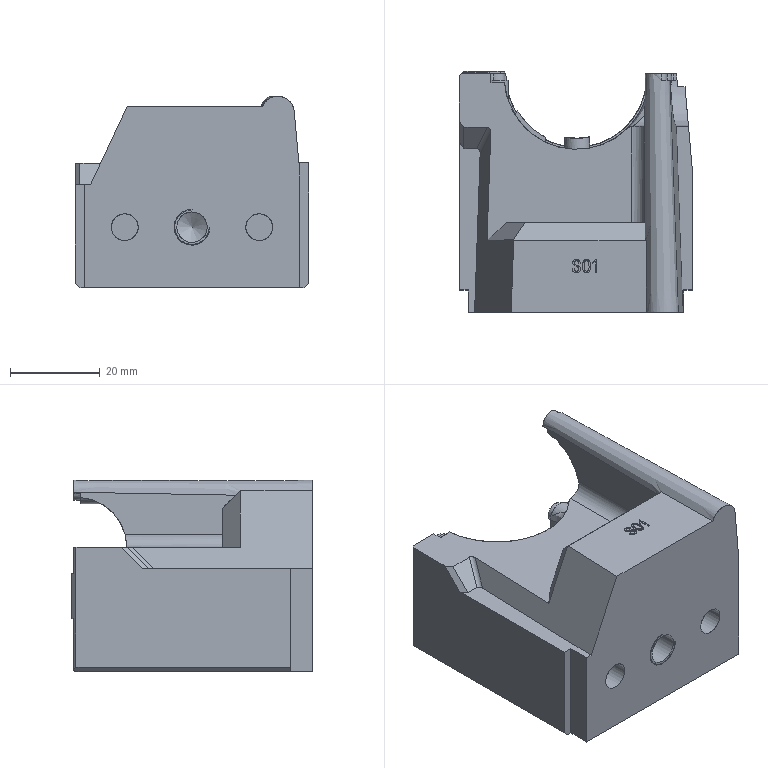NC program | PowerMill | posted with a generic post | part box 52 x 53.756 x 42.711 mm
Whole program:
%
O0001
N104 ( POWERMILL CB  : 2026004.0)
N105 ( POST VER      : 2026.0.0.5161)
N106 ( OPTION FILE   : FANUC)
N107 ( OUTPUT WORKPLANE : 1)
N108 (  )
N109 ( TOOL LIST )
N110 (--------------------------------)
N111 ( NO. | ID | DIA.| TIP RAD|LENGTH)
N112 (--------------------------------)
N113 (    1|D8_2| 8.0 |  0.0   | 99.0 )
N114 (--------------------------------)
N115 (  )
N116 ( NUMBER OF TOOLPATHS: 1.0 )
N117 ( ESTIMATED PROGRAM DURATION: 0 HOURS 1 MIN 35 SEC)
N118 (  )
N119 G00 G21 G80 G40 G17
N120 G90
N121 G54
N122 G53 Z0.0
N123 (---------------)
N124 ( START TOOLPATH : 02开粗-D8-等高 )
N125 (---------------)
N126 ( TOOL NO.    :1 )
N127 ( TOOL TYPE   : ENDMILL)
N128 ( TOOL ID     : D8_2)
N129 ( TOOL DIA    : 8.0 LENGTH 99.0)
N130 T1
N131 M6
N132 S3500 M03
N133 G00 G90 X28.2444 Y-5.4315
N134 G43 Z20.0 H1
N135
N136 G05 P10000 R8
N137 Z2.8808
N138 G01 Z-0.1192 F1680.0
N139 G02 X28.03 Y-4.6315 I1.3856 J0.8 F2800.0
N140 G01 Y0.1685
N141 Y42.5415
N142 Y47.3415
N143 G02 X28.2443 Y48.1415 I1.6 J0.0
N144 G01 X28.2654 Y48.178 Z-0.1366
N145 X28.2741 Y48.1931 Z-0.1788
N146 X28.2654 Y48.178 Z-0.2209
N147 X28.2443 Y48.1415 Z-0.2384
N148 G03 X28.03 Y47.3415 I1.3857 J-0.8
N149 G01 Y42.5415
N150 Y0.1685
N151 Y-4.6315
N152 G03 X28.2444 Y-5.4315 I1.6 J0.0
N153 G01 X28.2654 Y-5.468 Z-0.2558
N154 X28.2742 Y-5.4832 Z-0.298
N155 X28.2654 Y-5.468 Z-0.3401
N156 X28.2444 Y-5.4315 Z-0.3576
N157 G02 X28.03 Y-4.6315 I1.3856 J0.8
N158 G01 Y0.1685
N159 Y42.5415
N160 Y47.3415
N161 G02 X28.2443 Y48.1415 I1.6 J0.0
N162 G01 X28.2654 Y48.178 Z-0.375
N163 X28.2741 Y48.1931 Z-0.4172
N164 X28.2654 Y48.178 Z-0.4593
N165 X28.2443 Y48.1415 Z-0.4768
N166 G03 X28.03 Y47.3415 I1.3857 J-0.8
N167 G01 Y42.5415
N168 Y0.1685
N169 Y-4.6315
N170 G03 X28.2444 Y-5.4315 I1.6 J0.0
N171 G01 X28.2654 Y-5.468 Z-0.4942
N172 X28.2742 Y-5.4832 Z-0.5364
N173 X28.2654 Y-5.468 Z-0.5785
N174 X28.2444 Y-5.4315 Z-0.596
N175 G02 X28.03 Y-4.6315 I1.3856 J0.8
N176 G01 Y0.1685
N177 Y42.5415
N178 Y47.3415
N179 G02 X28.2443 Y48.1415 I1.6 J0.0
N180 G01 X28.2654 Y48.178 Z-0.6134
N181 X28.2741 Y48.1931 Z-0.6555
N182 X28.2654 Y48.178 Z-0.6977
N183 X28.2443 Y48.1415 Z-0.7151
N184 G03 X28.03 Y47.3415 I1.3857 J-0.8
N185 G01 Y42.5415
N186 Y0.1685
N187 Y-4.6315
N188 G03 X28.2444 Y-5.4315 I1.6 J0.0
N189 G01 X28.2654 Y-5.468 Z-0.7326
N190 X28.2742 Y-5.4832 Z-0.7747
N191 X28.2654 Y-5.468 Z-0.8169
N192 X28.2444 Y-5.4315 Z-0.8343
N193 G02 X28.03 Y-4.6315 I1.3856 J0.8
N194 G01 Y0.1685
N195 Y42.5415
N196 Y47.3415
N197 G02 X28.2443 Y48.1415 I1.6 J0.0
N198 G01 X28.2654 Y48.178 Z-0.8518
N199 X28.2741 Y48.1931 Z-0.8939
N200 X28.2654 Y48.178 Z-0.9361
N201 X28.2443 Y48.1415 Z-0.9535
N202 G03 X28.03 Y47.3415 I1.3857 J-0.8
N203 G01 Y42.5415
N204 Y0.1685
N205 Y-4.6315
N206 G03 X28.2444 Y-5.4315 I1.6 J0.0
N207 G01 X28.2654 Y-5.468 Z-0.971
N208 X28.2742 Y-5.4832 Z-1.0131
N209 X28.2654 Y-5.468 Z-1.0553
N210 X28.2444 Y-5.4315 Z-1.0727
N211 G02 X28.03 Y-4.6315 I1.3856 J0.8
N212 G01 Y0.1685
N213 Y42.5415
N214 Y47.3415
N215 G02 X28.2443 Y48.1415 I1.6 J0.0
N216 G01 X28.2654 Y48.178 Z-1.0902
N217 X28.2741 Y48.1931 Z-1.1323
N218 X28.2654 Y48.178 Z-1.1745
N219 X28.2443 Y48.1415 Z-1.1919
N220 G03 X28.03 Y47.3415 I1.3857 J-0.8
N221 G01 Y42.5415
N222 Y0.1685
N223 Y-4.6315
N224 G03 X28.2444 Y-5.4315 I1.6 J0.0
N225 G01 X28.2654 Y-5.468 Z-1.2094
N226 X28.2742 Y-5.4832 Z-1.2515
N227 X28.2654 Y-5.468 Z-1.2936
N228 X28.2444 Y-5.4315 Z-1.3111
N229 G02 X28.03 Y-4.6315 I1.3856 J0.8
N230 G01 Y0.1685
N231 Y42.5415
N232 Y47.3415
N233 G02 X28.2443 Y48.1415 I1.6 J0.0
N234 G01 X28.2654 Y48.178 Z-1.3285
N235 X28.2741 Y48.1931 Z-1.3707
N236 X28.2654 Y48.178 Z-1.4128
N237 X28.2443 Y48.1415 Z-1.4303
N238 G03 X28.03 Y47.3415 I1.3857 J-0.8
N239 G01 Y42.5415
N240 Y0.1685
N241 Y-4.6315
N242 G03 X28.2444 Y-5.4315 I1.6 J0.0
N243 G01 X28.2654 Y-5.468 Z-1.4477
N244 X28.2742 Y-5.4832 Z-1.4899
N245 X28.2654 Y-5.468 Z-1.532
N246 X28.2444 Y-5.4315 Z-1.5495
N247 G02 X28.03 Y-4.6315 I1.3856 J0.8
N248 G01 Y0.1685
N249 Y42.5415
N250 Y47.3415
N251 G02 X28.2443 Y48.1415 I1.6 J0.0
N252 G01 X28.2654 Y48.178 Z-1.5669
N253 X28.2741 Y48.1931 Z-1.6091
N254 X28.2654 Y48.178 Z-1.6512
N255 X28.2443 Y48.1415 Z-1.6687
N256 G03 X28.03 Y47.3415 I1.3857 J-0.8
N257 G01 Y42.5415
N258 Y0.1685
N259 Y-4.6315
N260 G03 X28.2444 Y-5.4315 I1.6 J0.0
N261 G01 X28.2654 Y-5.468 Z-1.6861
N262 X28.2742 Y-5.4832 Z-1.7283
N263 X28.2654 Y-5.468 Z-1.7704
N264 X28.2444 Y-5.4315 Z-1.7879
N265 G02 X28.03 Y-4.6315 I1.3856 J0.8
N266 G01 Y0.1685
N267 Y42.5415
N268 Y47.3415
N269 G02 X28.2443 Y48.1415 I1.6 J0.0
N270 G01 X28.2654 Y48.178 Z-1.8053
N271 X28.2741 Y48.1931 Z-1.8475
N272 X28.2654 Y48.178 Z-1.8896
N273 X28.2443 Y48.1415 Z-1.907
N274 G03 X28.03 Y47.3415 I1.3857 J-0.8
N275 G01 Y42.5415
N276 Y0.1685
N277 Y-4.6315
N278 G03 X28.2444 Y-5.4315 I1.6 J0.0
N279 G01 X28.2654 Y-5.468 Z-1.9245
N280 X28.2742 Y-5.4832 Z-1.9666
N281 X28.2654 Y-5.468 Z-2.0088
N282 X28.2444 Y-5.4315 Z-2.0262
N283 G02 X28.03 Y-4.6315 I1.3856 J0.8
N284 G01 Y0.1685
N285 Y42.5415
N286 Y47.3415
N287 G02 X28.2443 Y48.1415 I1.6 J0.0
N288 G01 X28.2654 Y48.178 Z-2.0437
N289 X28.2741 Y48.1931 Z-2.0858
N290 X28.2654 Y48.178 Z-2.128
N291 X28.2443 Y48.1415 Z-2.1454
N292 G03 X28.03 Y47.3415 I1.3857 J-0.8
N293 G01 Y42.5415
N294 Y0.1685
N295 Y-4.6315
N296 G03 X28.2444 Y-5.4315 I1.6 J0.0
N297 G01 X28.2654 Y-5.468 Z-2.1629
N298 X28.2742 Y-5.4832 Z-2.205
N299 X28.2654 Y-5.468 Z-2.2472
N300 X28.2444 Y-5.4315 Z-2.2646
N301 G02 X28.03 Y-4.6315 I1.3856 J0.8
N302 G01 Y0.1685
N303 Y42.5415
N304 Y47.3415
N305 G02 X28.2443 Y48.1415 I1.6 J0.0
N306 G01 X28.2654 Y48.178 Z-2.2821
N307 X28.2741 Y48.1931 Z-2.3242
N308 X28.2654 Y48.178 Z-2.3664
N309 X28.2443 Y48.1415 Z-2.3838
N310 G03 X28.03 Y47.3415 I1.3857 J-0.8
N311 G01 Y42.5415
N312 Y0.1685
N313 Y-4.6315
N314 G03 X28.2444 Y-5.4315 I1.6 J0.0
N315 G01 X28.2654 Y-5.468 Z-2.4013
N316 X28.2742 Y-5.4832 Z-2.4434
N317 X28.2655 Y-5.468 Z-2.4855
N318 X28.2444 Y-5.4315 Z-2.503
N319 G02 X28.03 Y-4.6315 I1.3856 J0.8
N320 G01 Y0.1685
N321 Y42.5415
N322 Y47.3415
N323 G02 X28.2443 Y48.1415 I1.6 J0.0
N324 G01 X28.2654 Y48.178 Z-2.5205
N325 X28.2741 Y48.1931 Z-2.5626
N326 X28.2654 Y48.178 Z-2.6047
N327 X28.2443 Y48.1415 Z-2.6222
N328 G03 X28.03 Y47.3415 I1.3857 J-0.8
N329 G01 Y42.5415
N330 Y0.1685
N331 Y-4.6315
N332 G03 X28.2444 Y-5.4315 I1.6 J0.0
N333 G01 X28.2655 Y-5.468 Z-2.6396
N334 X28.2742 Y-5.4832 Z-2.6818
N335 X28.2655 Y-5.468 Z-2.7239
N336 X28.2444 Y-5.4315 Z-2.7414
N337 G02 X28.03 Y-4.6315 I1.3856 J0.8
N338 G01 Y0.1685
N339 Y42.5415
N340 Y47.3415
N341 G02 X28.2444 Y48.1415 I1.6 J0.0
N342 G01 X28.2654 Y48.178 Z-2.7588
N343 X28.2741 Y48.1931 Z-2.801
N344 X28.2654 Y48.178 Z-2.8431
N345 X28.2444 Y48.1415 Z-2.8606
N346 G03 X28.03 Y47.3415 I1.3856 J-0.8
N347 G01 Y42.5415
N348 Y0.1685
N349 Y-4.6315
N350 G03 X28.2444 Y-5.4315 I1.6 J0.0
N351 G01 X28.2655 Y-5.468 Z-2.878
N352 X28.2742 Y-5.4832 Z-2.9202
N353 X28.2655 Y-5.468 Z-2.9623
N354 X28.2444 Y-5.4315 Z-2.9798
N355 G02 X28.03 Y-4.6315 I1.3856 J0.8
N356 G01 Y0.1685
N357 Y42.5415
N358 Y47.3415
N359 G02 X28.2444 Y48.1415 I1.6 J0.0
N360 G01 X28.2654 Y48.178 Z-2.9972
N361 X28.2742 Y48.1931 Z-3.0394
N362 X28.2654 Y48.178 Z-3.0815
N363 X28.2444 Y48.1415 Z-3.099
N364 G03 X28.03 Y47.3415 I1.3856 J-0.8
N365 G01 Y42.5415
N366 Y0.1685
N367 Y-4.6315
N368 G03 X28.2444 Y-5.4315 I1.6 J0.0
N369 G01 X28.2655 Y-5.468 Z-3.1164
N370 X28.2742 Y-5.4832 Z-3.1585
N371 X28.2655 Y-5.468 Z-3.2007
N372 X28.2444 Y-5.4315 Z-3.2181
N373 G02 X28.03 Y-4.6315 I1.3856 J0.8
N374 G01 Y0.1685
N375 Y42.5415
N376 Y47.3415
N377 G02 X28.2444 Y48.1415 I1.6 J0.0
N378 G01 X28.2654 Y48.178 Z-3.2356
N379 X28.2742 Y48.1932 Z-3.2777
N380 X28.2654 Y48.178 Z-3.3199
N381 X28.2444 Y48.1415 Z-3.3373
N382 G03 X28.03 Y47.3415 I1.3856 J-0.8
N383 G01 Y42.5415
N384 Y0.1685
N385 Y-4.6315
N386 G03 X28.2444 Y-5.4315 I1.6 J0.0
N387 G01 X28.2655 Y-5.468 Z-3.3548
N388 X28.2742 Y-5.4832 Z-3.3969
N389 X28.2655 Y-5.468 Z-3.4391
N390 X28.2444 Y-5.4315 Z-3.4565
N391 G02 X28.03 Y-4.6315 I1.3856 J0.8
N392 G01 Y0.1685
N393 Y42.5415
N394 Y47.3415
N395 G02 X28.2444 Y48.1415 I1.6 J0.0
N396 G01 X28.2654 Y48.178 Z-3.474
N397 X28.2742 Y48.1931 Z-3.5161
N398 X28.2654 Y48.178 Z-3.5583
N399 X28.2444 Y48.1415 Z-3.5757
N400 G03 X28.03 Y47.3415 I1.3856 J-0.8
N401 G01 Y42.5415
N402 Y0.1685
N403 Y-4.6315
N404 G03 X28.2444 Y-5.4315 I1.6 J0.0
N405 G01 X28.2655 Y-5.468 Z-3.5932
N406 X28.2742 Y-5.4832 Z-3.6353
N407 X28.2655 Y-5.468 Z-3.6774
N408 X28.2444 Y-5.4315 Z-3.6949
N409 G02 X28.03 Y-4.6315 I1.3856 J0.8
N410 G01 Y0.1685
N411 Y42.5415
N412 Y47.3415
N413 G02 X28.2444 Y48.1415 I1.6 J0.0
N414 G01 X28.2654 Y48.178 Z-3.7124
N415 X28.2742 Y48.1931 Z-3.7545
N416 X28.2654 Y48.178 Z-3.7966
N417 X28.2444 Y48.1415 Z-3.8141
N418 G03 X28.03 Y47.3415 I1.3856 J-0.8
N419 G01 Y42.5415
N420 Y0.1685
N421 Y-4.6315
N422 G03 X28.2444 Y-5.4315 I1.6 J0.0
N423 G01 X28.2655 Y-5.468 Z-3.8316
N424 X28.2742 Y-5.4832 Z-3.8737
N425 X28.2655 Y-5.468 Z-3.9158
N426 X28.2444 Y-5.4315 Z-3.9333
N427 G02 X28.03 Y-4.6315 I1.3856 J0.8
N428 G01 Y0.1685
N429 Y42.5415
N430 Y47.3415
N431 G02 X28.2444 Y48.1415 I1.6 J0.0
N432 G01 X28.2654 Y48.178 Z-3.9507
N433 X28.2742 Y48.1932 Z-3.9929
N434 X28.2654 Y48.178 Z-4.035
N435 X28.2444 Y48.1415 Z-4.0525
N436 G03 X28.03 Y47.3415 I1.3856 J-0.8
N437 G01 Y42.5415
N438 Y0.1685
N439 Y-4.6315
N440 G03 X28.2444 Y-5.4315 I1.6 J0.0
N441 G01 X28.2655 Y-5.468 Z-4.0699
N442 X28.2742 Y-5.4832 Z-4.1121
N443 X28.2655 Y-5.468 Z-4.1542
N444 X28.2444 Y-5.4315 Z-4.1717
N445 G02 X28.03 Y-4.6315 I1.3856 J0.8
N446 G01 Y0.1685
N447 Y42.5415
N448 Y47.3415
N449 G02 X28.2444 Y48.1415 I1.6 J0.0
N450 G01 X28.2654 Y48.178 Z-4.1891
N451 X28.2742 Y48.1932 Z-4.2313
N452 X28.2654 Y48.178 Z-4.2734
N453 X28.2444 Y48.1415 Z-4.2909
N454 G03 X28.03 Y47.3415 I1.3856 J-0.8
N455 G01 Y42.5415
N456 Y0.1685
N457 Y-4.6315
N458 G03 X28.2444 Y-5.4315 I1.6 J0.0
N459 G01 X28.2655 Y-5.468 Z-4.3083
N460 X28.2742 Y-5.4832 Z-4.3505
N461 X28.2655 Y-5.468 Z-4.3926
N462 X28.2444 Y-5.4315 Z-4.41
N463 G02 X28.03 Y-4.6315 I1.3856 J0.8
N464 G01 Y0.1685
N465 Y42.5415
N466 Y47.3415
N467 G02 X28.2444 Y48.1415 I1.6 J0.0
N468 G01 X28.2654 Y48.178 Z-4.4275
N469 X28.2742 Y48.1932 Z-4.4696
N470 X28.2654 Y48.178 Z-4.5118
N471 X28.2444 Y48.1415 Z-4.5292
N472 G03 X28.03 Y47.3415 I1.3856 J-0.8
N473 G01 Y42.5415
N474 Y0.1685
N475 Y-4.6315
N476 G03 X28.2444 Y-5.4315 I1.6 J0.0
N477 G01 X28.2655 Y-5.468 Z-4.5467
N478 X28.2742 Y-5.4832 Z-4.5888
N479 X28.2655 Y-5.468 Z-4.631
N480 X28.2444 Y-5.4315 Z-4.6484
N481 G02 X28.03 Y-4.6315 I1.3856 J0.8
N482 G01 Y0.1685
N483 Y42.5415
N484 Y47.3415
N485 G02 X28.2444 Y48.1415 I1.6 J0.0
N486 G01 X28.2654 Y48.178 Z-4.6659
N487 X28.2742 Y48.1932 Z-4.708
N488 X28.2654 Y48.178 Z-4.7502
N489 X28.2444 Y48.1415 Z-4.7676
N490 G03 X28.03 Y47.3415 I1.3856 J-0.8
N491 G01 Y42.5415
N492 Y0.1685
N493 Y-4.6315
N494 G03 X28.2444 Y-5.4315 I1.6 J0.0
N495 G01 X28.2655 Y-5.468 Z-4.7851
N496 X28.2742 Y-5.4832 Z-4.8272
N497 X28.2655 Y-5.468 Z-4.8694
N498 X28.2444 Y-5.4315 Z-4.8868
N499 G02 X28.03 Y-4.6315 I1.3856 J0.8
N500 G01 Y0.1685
N501 Y42.5415
N502 Y47.3415
N503 G02 X28.2444 Y48.1415 I1.6 J0.0
N504 G00 Z5.2882
N505 G01 X-28.2443 Y-5.4315 F10000.0
N506 G00 Z2.8808
N507 G01 Z-0.1192 F1680.0
N508 G03 X-28.03 Y-4.6315 I-1.3857 J0.8 F2800.0
N509 G01 Y0.1685
N510 Y42.5415
N511 Y47.3415
N512 G03 X-28.2443 Y48.1415 I-1.5999 J0.0001
N513 G01 X-28.2654 Y48.178 Z-0.1366
N514 X-28.2741 Y48.1931 Z-0.1788
N515 X-28.2654 Y48.178 Z-0.2209
N516 X-28.2443 Y48.1415 Z-0.2384
N517 G02 X-28.03 Y47.3415 I-1.3856 J-0.7999
N518 G01 Y42.5415
N519 Y0.1685
N520 Y-4.6315
N521 G02 X-28.2443 Y-5.4315 I-1.6 J0.0
N522 G01 X-28.2654 Y-5.468 Z-0.2558
N523 X-28.2741 Y-5.4832 Z-0.298
N524 X-28.2654 Y-5.468 Z-0.3401
N525 X-28.2443 Y-5.4315 Z-0.3576
N526 G03 X-28.03 Y-4.6315 I-1.3857 J0.8
N527 G01 Y0.1685
N528 Y42.5415
N529 Y47.3415
N530 G03 X-28.2443 Y48.1415 I-1.5999 J0.0001
N531 G01 X-28.2654 Y48.178 Z-0.375
N532 X-28.2741 Y48.1931 Z-0.4172
N533 X-28.2654 Y48.178 Z-0.4593
N534 X-28.2443 Y48.1415 Z-0.4768
N535 G02 X-28.03 Y47.3415 I-1.3856 J-0.7999
N536 G01 Y42.5415
N537 Y0.1685
N538 Y-4.6315
N539 G02 X-28.2443 Y-5.4315 I-1.6 J0.0
N540 G01 X-28.2654 Y-5.468 Z-0.4942
N541 X-28.2741 Y-5.4832 Z-0.5364
N542 X-28.2654 Y-5.468 Z-0.5785
N543 X-28.2443 Y-5.4315 Z-0.596
N544 G03 X-28.03 Y-4.6315 I-1.3857 J0.8
N545 G01 Y0.1685
N546 Y42.5415
N547 Y47.3415
N548 G03 X-28.2443 Y48.1415 I-1.5999 J0.0001
N549 G01 X-28.2654 Y48.178 Z-0.6134
N550 X-28.2741 Y48.1931 Z-0.6555
N551 X-28.2654 Y48.178 Z-0.6977
N552 X-28.2443 Y48.1415 Z-0.7151
N553 G02 X-28.03 Y47.3415 I-1.3856 J-0.7999
N554 G01 Y42.5415
N555 Y0.1685
N556 Y-4.6315
N557 G02 X-28.2443 Y-5.4315 I-1.6 J0.0
N558 G01 X-28.2654 Y-5.468 Z-0.7326
N559 X-28.2741 Y-5.4832 Z-0.7747
N560 X-28.2654 Y-5.468 Z-0.8169
N561 X-28.2443 Y-5.4315 Z-0.8343
N562 G03 X-28.03 Y-4.6315 I-1.3857 J0.8
N563 G01 Y0.1685
N564 Y42.5415
N565 Y47.3415
N566 G03 X-28.2443 Y48.1415 I-1.5999 J0.0001
N567 G01 X-28.2654 Y48.178 Z-0.8518
N568 X-28.2741 Y48.1931 Z-0.8939
N569 X-28.2654 Y48.178 Z-0.9361
N570 X-28.2443 Y48.1415 Z-0.9535
N571 G02 X-28.03 Y47.3415 I-1.3856 J-0.7999
N572 G01 Y42.5415
N573 Y0.1685
N574 Y-4.6315
N575 G02 X-28.2443 Y-5.4315 I-1.6 J0.0
N576 G01 X-28.2654 Y-5.468 Z-0.971
N577 X-28.2741 Y-5.4832 Z-1.0131
N578 X-28.2654 Y-5.468 Z-1.0553
N579 X-28.2443 Y-5.4315 Z-1.0727
N580 G03 X-28.03 Y-4.6315 I-1.3857 J0.8
N581 G01 Y0.1685
N582 Y42.5415
N583 Y47.3415
N584 G03 X-28.2443 Y48.1415 I-1.5999 J0.0001
N585 G01 X-28.2654 Y48.178 Z-1.0902
N586 X-28.2741 Y48.1931 Z-1.1323
N587 X-28.2654 Y48.178 Z-1.1745
N588 X-28.2443 Y48.1415 Z-1.1919
N589 G02 X-28.03 Y47.3415 I-1.3856 J-0.7999
N590 G01 Y42.5415
N591 Y0.1685
N592 Y-4.6315
N593 G02 X-28.2443 Y-5.4315 I-1.6 J0.0
N594 G01 X-28.2654 Y-5.468 Z-1.2094
N595 X-28.2741 Y-5.4832 Z-1.2515
N596 X-28.2654 Y-5.468 Z-1.2936
N597 X-28.2444 Y-5.4315 Z-1.3111
N598 G03 X-28.03 Y-4.6315 I-1.3856 J0.8
N599 G01 Y0.1685
N600 Y42.5415
N601 Y47.3415
N602 G03 X-28.2444 Y48.1415 I-1.5999 J0.0001
N603 G01 X-28.2654 Y48.178 Z-1.3285
N604 X-28.2741 Y48.1931 Z-1.3707
N605 X-28.2654 Y48.178 Z-1.4128
N606 X-28.2444 Y48.1415 Z-1.4303
N607 G02 X-28.03 Y47.3415 I-1.3855 J-0.7999
N608 G01 Y42.5415
N609 Y0.1685
N610 Y-4.6315
N611 G02 X-28.2444 Y-5.4315 I-1.6 J0.0
N612 G01 X-28.2654 Y-5.468 Z-1.4477
N613 X-28.2741 Y-5.4832 Z-1.4899
N614 X-28.2654 Y-5.468 Z-1.532
N615 X-28.2444 Y-5.4315 Z-1.5495
N616 G03 X-28.03 Y-4.6315 I-1.3856 J0.8
N617 G01 Y0.1685
N618 Y42.5415
N619 Y47.3415
N620 G03 X-28.2444 Y48.1415 I-1.6 J0.0001
N621 G01 X-28.2654 Y48.178 Z-1.5669
N622 X-28.2742 Y48.1931 Z-1.6091
N623 X-28.2654 Y48.178 Z-1.6512
N624 X-28.2444 Y48.1415 Z-1.6687
N625 G02 X-28.03 Y47.3415 I-1.3856 J-0.7999
N626 G01 Y42.5415
N627 Y0.1685
N628 Y-4.6315
N629 G02 X-28.2444 Y-5.4315 I-1.6 J0.0
N630 G01 X-28.2654 Y-5.468 Z-1.6861
N631 X-28.2742 Y-5.4832 Z-1.7283
N632 X-28.2654 Y-5.468 Z-1.7704
N633 X-28.2444 Y-5.4315 Z-1.7879
N634 G03 X-28.03 Y-4.6315 I-1.3856 J0.8
N635 G01 Y0.1685
N636 Y42.5415
N637 Y47.3415
N638 G03 X-28.2444 Y48.1415 I-1.6 J0.0001
N639 G01 X-28.2654 Y48.178 Z-1.8053
N640 X-28.2742 Y48.1931 Z-1.8475
N641 X-28.2654 Y48.178 Z-1.8896
N642 X-28.2444 Y48.1415 Z-1.907
N643 G02 X-28.03 Y47.3415 I-1.3856 J-0.7999
N644 G01 Y42.5415
N645 Y0.1685
N646 Y-4.6315
N647 G02 X-28.2444 Y-5.4315 I-1.6 J0.0
N648 G01 X-28.2654 Y-5.468 Z-1.9245
N649 X-28.2742 Y-5.4832 Z-1.9666
N650 X-28.2654 Y-5.468 Z-2.0088
N651 X-28.2444 Y-5.4315 Z-2.0262
N652 G03 X-28.03 Y-4.6315 I-1.3856 J0.8
N653 G01 Y0.1685
N654 Y42.5415
N655 Y47.3415
N656 G03 X-28.2444 Y48.1415 I-1.6 J0.0001
N657 G01 X-28.2654 Y48.178 Z-2.0437
N658 X-28.2742 Y48.1931 Z-2.0858
N659 X-28.2654 Y48.178 Z-2.128
N660 X-28.2444 Y48.1415 Z-2.1454
N661 G02 X-28.03 Y47.3415 I-1.3856 J-0.7999
N662 G01 Y42.5415
N663 Y0.1685
N664 Y-4.6315
N665 G02 X-28.2444 Y-5.4315 I-1.6 J0.0
N666 G01 X-28.2654 Y-5.468 Z-2.1629
N667 X-28.2742 Y-5.4832 Z-2.205
N668 X-28.2654 Y-5.468 Z-2.2472
N669 X-28.2444 Y-5.4315 Z-2.2646
N670 G03 X-28.03 Y-4.6315 I-1.3856 J0.8
N671 G01 Y0.1685
N672 Y42.5415
N673 Y47.3415
N674 G03 X-28.2444 Y48.1415 I-1.6 J0.0001
N675 G01 X-28.2654 Y48.178 Z-2.2821
N676 X-28.2742 Y48.1931 Z-2.3242
N677 X-28.2654 Y48.178 Z-2.3664
N678 X-28.2444 Y48.1415 Z-2.3838
N679 G02 X-28.03 Y47.3415 I-1.3856 J-0.7999
N680 G01 Y42.5415
N681 Y0.1685
N682 Y-4.6315
N683 G02 X-28.2444 Y-5.4315 I-1.6 J0.0
N684 G01 X-28.2654 Y-5.468 Z-2.4013
N685 X-28.2742 Y-5.4832 Z-2.4434
N686 X-28.2654 Y-5.468 Z-2.4855
N687 X-28.2444 Y-5.4315 Z-2.503
N688 G03 X-28.03 Y-4.6315 I-1.3856 J0.8
N689 G01 Y0.1685
N690 Y42.5415
N691 Y47.3415
N692 G03 X-28.2444 Y48.1415 I-1.6 J0.0001
N693 G01 X-28.2654 Y48.178 Z-2.5205
N694 X-28.2742 Y48.1931 Z-2.5626
N695 X-28.2654 Y48.178 Z-2.6047
N696 X-28.2444 Y48.1415 Z-2.6222
N697 G02 X-28.03 Y47.3415 I-1.3856 J-0.7999
N698 G01 Y42.5415
N699 Y0.1685
N700 Y-4.6315
N701 G02 X-28.2444 Y-5.4315 I-1.6 J0.0
N702 G01 X-28.2654 Y-5.468 Z-2.6396
N703 X-28.2742 Y-5.4832 Z-2.6818
N704 X-28.2654 Y-5.468 Z-2.7239
N705 X-28.2444 Y-5.4315 Z-2.7414
N706 G03 X-28.03 Y-4.6315 I-1.3856 J0.8
N707 G01 Y0.1685
N708 Y42.5415
N709 Y47.3415
N710 G03 X-28.2444 Y48.1415 I-1.6 J0.0001
N711 G01 X-28.2654 Y48.178 Z-2.7588
N712 X-28.2742 Y48.1931 Z-2.801
N713 X-28.2654 Y48.178 Z-2.8431
N714 X-28.2444 Y48.1415 Z-2.8606
N715 G02 X-28.03 Y47.3415 I-1.3856 J-0.7999
N716 G01 Y42.5415
N717 Y0.1685
N718 Y-4.6315
N719 G02 X-28.2444 Y-5.4315 I-1.6 J0.0
N720 G01 X-28.2654 Y-5.468 Z-2.878
N721 X-28.2742 Y-5.4832 Z-2.9202
N722 X-28.2654 Y-5.468 Z-2.9623
N723 X-28.2444 Y-5.4315 Z-2.9798
N724 G03 X-28.03 Y-4.6315 I-1.3856 J0.8
N725 G01 Y0.1685
N726 Y42.5415
N727 Y47.3415
N728 G03 X-28.2444 Y48.1415 I-1.6 J0.0001
N729 G01 X-28.2654 Y48.178 Z-2.9972
N730 X-28.2742 Y48.1931 Z-3.0394
N731 X-28.2654 Y48.178 Z-3.0815
N732 X-28.2444 Y48.1415 Z-3.099
N733 G02 X-28.03 Y47.3415 I-1.3856 J-0.7999
N734 G01 Y42.5415
N735 Y0.1685
N736 Y-4.6315
N737 G02 X-28.2444 Y-5.4315 I-1.6 J0.0
N738 G01 X-28.2654 Y-5.468 Z-3.1164
N739 X-28.2742 Y-5.4832 Z-3.1585
N740 X-28.2654 Y-5.468 Z-3.2007
N741 X-28.2444 Y-5.4315 Z-3.2181
N742 G03 X-28.03 Y-4.6315 I-1.3856 J0.8
N743 G01 Y0.1685
N744 Y42.5415
N745 Y47.3415
N746 G03 X-28.2444 Y48.1415 I-1.6 J0.0001
N747 G01 X-28.2654 Y48.178 Z-3.2356
N748 X-28.2742 Y48.1931 Z-3.2777
N749 X-28.2654 Y48.178 Z-3.3199
N750 X-28.2444 Y48.1415 Z-3.3373
N751 G02 X-28.03 Y47.3415 I-1.3856 J-0.7999
N752 G01 Y42.5415
N753 Y0.1685
N754 Y-4.6315
N755 G02 X-28.2444 Y-5.4315 I-1.6 J0.0
N756 G01 X-28.2654 Y-5.468 Z-3.3548
N757 X-28.2742 Y-5.4832 Z-3.3969
N758 X-28.2654 Y-5.468 Z-3.4391
N759 X-28.2444 Y-5.4315 Z-3.4565
N760 G03 X-28.03 Y-4.6315 I-1.3856 J0.8
N761 G01 Y0.1685
N762 Y42.5415
N763 Y47.3415
N764 G03 X-28.2444 Y48.1415 I-1.6 J0.0001
N765 G01 X-28.2654 Y48.178 Z-3.474
N766 X-28.2742 Y48.1931 Z-3.5161
N767 X-28.2654 Y48.178 Z-3.5583
N768 X-28.2444 Y48.1415 Z-3.5757
N769 G02 X-28.03 Y47.3415 I-1.3856 J-0.7999
N770 G01 Y42.5415
N771 Y0.1685
N772 Y-4.6315
N773 G02 X-28.2444 Y-5.4315 I-1.6 J0.0
N774 G01 X-28.2654 Y-5.468 Z-3.5932
N775 X-28.2742 Y-5.4832 Z-3.6353
N776 X-28.2654 Y-5.468 Z-3.6774
N777 X-28.2444 Y-5.4315 Z-3.6949
N778 G03 X-28.03 Y-4.6315 I-1.3856 J0.8
N779 G01 Y0.1685
N780 Y42.5415
N781 Y47.3415
N782 G03 X-28.2444 Y48.1415 I-1.6 J0.0001
N783 G01 X-28.2654 Y48.178 Z-3.7124
N784 X-28.2742 Y48.1931 Z-3.7545
N785 X-28.2654 Y48.178 Z-3.7966
N786 X-28.2444 Y48.1415 Z-3.8141
N787 G02 X-28.03 Y47.3415 I-1.3856 J-0.7999
N788 G01 Y42.5415
N789 Y0.1685
N790 Y-4.6315
N791 G02 X-28.2444 Y-5.4315 I-1.6 J0.0
N792 G01 X-28.2654 Y-5.468 Z-3.8316
N793 X-28.2742 Y-5.4832 Z-3.8737
N794 X-28.2654 Y-5.468 Z-3.9158
N795 X-28.2444 Y-5.4315 Z-3.9333
N796 G03 X-28.03 Y-4.6315 I-1.3856 J0.8
N797 G01 Y0.1685
N798 Y42.5415
N799 Y47.3415
N800 G03 X-28.2444 Y48.1415 I-1.6 J0.0001
N801 G01 X-28.2654 Y48.178 Z-3.9507
N802 X-28.2742 Y48.1931 Z-3.9929
N803 X-28.2654 Y48.178 Z-4.035
N804 X-28.2444 Y48.1415 Z-4.0525
N805 G02 X-28.03 Y47.3415 I-1.3856 J-0.7999
N806 G01 Y42.5415
N807 Y0.1685
N808 Y-4.6315
N809 G02 X-28.2444 Y-5.4315 I-1.6 J0.0
N810 G01 X-28.2654 Y-5.468 Z-4.0699
N811 X-28.2742 Y-5.4832 Z-4.1121
N812 X-28.2654 Y-5.468 Z-4.1542
N813 X-28.2444 Y-5.4315 Z-4.1717
N814 G03 X-28.03 Y-4.6315 I-1.3856 J0.8
N815 G01 Y0.1685
N816 Y42.5415
N817 Y47.3415
N818 G03 X-28.2444 Y48.1415 I-1.6 J0.0001
N819 G01 X-28.2654 Y48.178 Z-4.1891
N820 X-28.2742 Y48.1931 Z-4.2313
N821 X-28.2654 Y48.178 Z-4.2734
N822 X-28.2444 Y48.1415 Z-4.2909
N823 G02 X-28.03 Y47.3415 I-1.3856 J-0.7999
N824 G01 Y42.5415
N825 Y0.1685
N826 Y-4.6315
N827 G02 X-28.2444 Y-5.4315 I-1.6 J0.0
N828 G01 X-28.2654 Y-5.468 Z-4.3083
N829 X-28.2742 Y-5.4832 Z-4.3505
N830 X-28.2654 Y-5.468 Z-4.3926
N831 X-28.2444 Y-5.4315 Z-4.41
N832 G03 X-28.03 Y-4.6315 I-1.3856 J0.8
N833 G01 Y0.1685
N834 Y42.5415
N835 Y47.3415
N836 G03 X-28.2444 Y48.1415 I-1.6 J0.0001
N837 G01 X-28.2654 Y48.178 Z-4.4275
N838 X-28.2742 Y48.1931 Z-4.4696
N839 X-28.2654 Y48.178 Z-4.5118
N840 X-28.2444 Y48.1415 Z-4.5292
N841 G02 X-28.03 Y47.3415 I-1.3856 J-0.7999
N842 G01 Y42.5415
N843 Y0.1685
N844 Y-4.6315
N845 G02 X-28.2444 Y-5.4315 I-1.6 J0.0
N846 G01 X-28.2654 Y-5.468 Z-4.5467
N847 X-28.2742 Y-5.4832 Z-4.5888
N848 X-28.2654 Y-5.468 Z-4.631
N849 X-28.2444 Y-5.4315 Z-4.6484
N850 G03 X-28.03 Y-4.6315 I-1.3856 J0.8
N851 G01 Y0.1685
N852 Y42.5415
N853 Y47.3415
N854 G03 X-28.2444 Y48.1415 I-1.6 J0.0001
N855 G01 X-28.2654 Y48.178 Z-4.6659
N856 X-28.2742 Y48.1931 Z-4.708
N857 X-28.2654 Y48.178 Z-4.7502
N858 X-28.2444 Y48.1415 Z-4.7676
N859 G02 X-28.03 Y47.3415 I-1.3856 J-0.7999
N860 G01 Y42.5415
N861 Y0.1685
N862 Y-4.6315
N863 G02 X-28.2444 Y-5.4315 I-1.6 J0.0
N864 G01 X-28.2654 Y-5.468 Z-4.7851
N865 X-28.2742 Y-5.4832 Z-4.8272
N866 X-28.2654 Y-5.468 Z-4.8694
N867 X-28.2444 Y-5.4315 Z-4.8868
N868 G03 X-28.03 Y-4.6315 I-1.3856 J0.8
N869 G01 Y0.1685
N870 Y42.5415
N871 Y47.3415
N872 G03 X-28.2444 Y48.1415 I-1.6 J0.0001
N873 G00 Z20.0
N874 G05 P0
N875 (---------------)
N876 ( END TOOLPATH : 02开粗-D8-等高 )
N877 (---------------)
N878
N879 M05
N880 G53 Z0.0
N881 M30
%